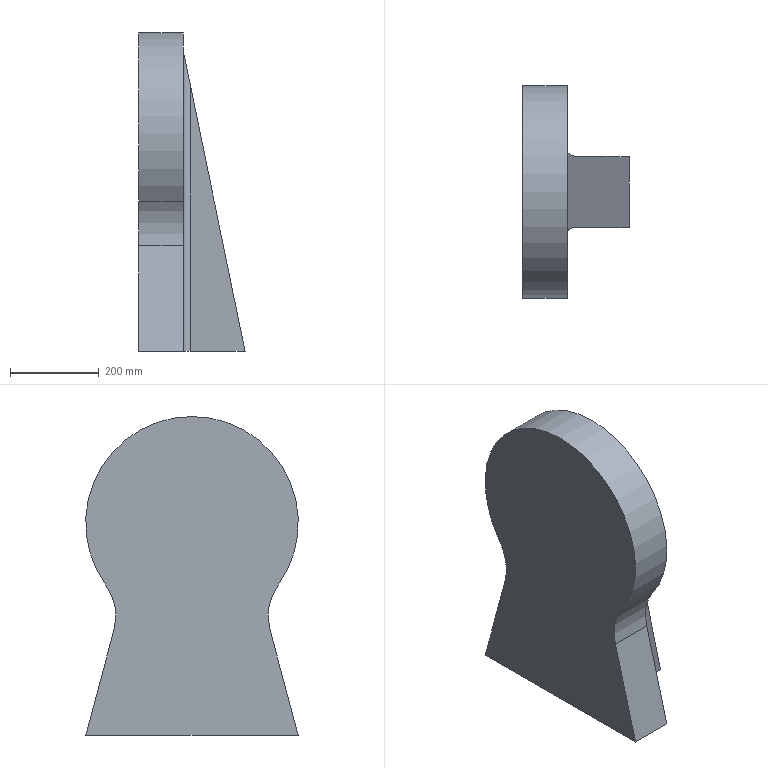Part | NX | features DATUM_CSYS 3, BLEND 2, EXTRUDE 2, SKETCH 2, CYLINDER 1 | 1 solid | 14 faces | box 240 x 480 x 720 mm | volume 36580765 mm3 | plane 8 | cylinder 6 | commonest cylinder face diameters 32 x3 240 x2 480 x1
STEP:
#1=CARTESIAN_POINT('',(100.,-96.,681.63));
#2=VERTEX_POINT('',#1);
#3=CARTESIAN_POINT('',(100.,96.,681.63));
#4=VERTEX_POINT('',#3);
#5=CARTESIAN_POINT('',(100.,0.,681.63));
#6=DIRECTION('',(0.,1.,0.));
#7=VECTOR('',#6,1000.);
#8=LINE('',#5,#7);
#9=EDGE_CURVE('',#2,#4,#8,.T.);
#10=ORIENTED_EDGE('',*,*,#9,.T.);
#11=CARTESIAN_POINT('',(100.,96.,0.));
#12=VERTEX_POINT('',#11);
#13=CARTESIAN_POINT('',(100.,96.,0.));
#14=DIRECTION('',(0.,0.,-1.));
#15=VECTOR('',#14,1000.);
#16=LINE('',#13,#15);
#17=EDGE_CURVE('',#4,#12,#16,.T.);
#18=ORIENTED_EDGE('',*,*,#17,.T.);
#19=CARTESIAN_POINT('',(100.,240.,0.));
#20=VERTEX_POINT('',#19);
#21=CARTESIAN_POINT('',(100.,-240.,0.));
#22=DIRECTION('',(0.,1.,0.));
#23=VECTOR('',#22,1000.);
#24=LINE('',#21,#23);
#25=EDGE_CURVE('',#12,#20,#24,.T.);
#26=ORIENTED_EDGE('',*,*,#25,.T.);
#27=CARTESIAN_POINT('',(100.,176.116,238.418));
#28=VERTEX_POINT('',#27);
#29=CARTESIAN_POINT('',(100.,240.,0.));
#30=DIRECTION('',(0.,-0.2588,0.9659));
#31=VECTOR('',#30,1000.);
#32=LINE('',#29,#31);
#33=EDGE_CURVE('',#20,#28,#32,.T.);
#34=ORIENTED_EDGE('',*,*,#33,.T.);
#35=CARTESIAN_POINT('',(100.,194.685,339.651));
#36=VERTEX_POINT('',#35);
#37=CARTESIAN_POINT('',(100.,292.027,269.476));
#38=DIRECTION('',(1.,0.,0.));
#39=DIRECTION('',(0.,0.,-1.));
#40=AXIS2_PLACEMENT_3D('',#37,#38,#39);
#41=CIRCLE('',#40,120.);
#42=EDGE_CURVE('',#28,#36,#41,.F.);
#43=ORIENTED_EDGE('',*,*,#42,.T.);
#44=CARTESIAN_POINT('',(100.,-194.685,339.651));
#45=VERTEX_POINT('',#44);
#46=CARTESIAN_POINT('',(100.,0.,480.));
#47=DIRECTION('',(-1.,0.,0.));
#48=DIRECTION('',(0.,0.,1.));
#49=AXIS2_PLACEMENT_3D('',#46,#47,#48);
#50=CIRCLE('',#49,240.);
#51=EDGE_CURVE('',#45,#36,#50,.T.);
#52=ORIENTED_EDGE('',*,*,#51,.F.);
#53=CARTESIAN_POINT('',(100.,-176.116,238.418));
#54=VERTEX_POINT('',#53);
#55=CARTESIAN_POINT('',(100.,-292.027,269.476));
#56=DIRECTION('',(1.,0.,0.));
#57=DIRECTION('',(0.,0.,-1.));
#58=AXIS2_PLACEMENT_3D('',#55,#56,#57);
#59=CIRCLE('',#58,120.);
#60=EDGE_CURVE('',#45,#54,#59,.F.);
#61=ORIENTED_EDGE('',*,*,#60,.T.);
#62=CARTESIAN_POINT('',(100.,-240.,0.));
#63=VERTEX_POINT('',#62);
#64=CARTESIAN_POINT('',(100.,-111.384,480.));
#65=DIRECTION('',(0.,-0.2588,-0.9659));
#66=VECTOR('',#65,1000.);
#67=LINE('',#64,#66);
#68=EDGE_CURVE('',#54,#63,#67,.T.);
#69=ORIENTED_EDGE('',*,*,#68,.T.);
#70=CARTESIAN_POINT('',(100.,-96.,0.));
#71=VERTEX_POINT('',#70);
#72=CARTESIAN_POINT('',(100.,-240.,0.));
#73=DIRECTION('',(0.,1.,0.));
#74=VECTOR('',#73,1000.);
#75=LINE('',#72,#74);
#76=EDGE_CURVE('',#63,#71,#75,.T.);
#77=ORIENTED_EDGE('',*,*,#76,.T.);
#78=CARTESIAN_POINT('',(100.,-96.,680.));
#79=DIRECTION('',(0.,0.,-1.));
#80=VECTOR('',#79,1000.);
#81=LINE('',#78,#80);
#82=EDGE_CURVE('',#71,#2,#81,.F.);
#83=ORIENTED_EDGE('',*,*,#82,.T.);
#84=EDGE_LOOP('',(#10,#18,#26,#34,#43,#52,#61,#69,#77,#83));
#85=FACE_BOUND('',#84,.T.);
#86=CARTESIAN_POINT('',(100.,0.,0.));
#87=DIRECTION('',(1.,0.,0.));
#88=DIRECTION('',(0.,0.,-1.));
#89=AXIS2_PLACEMENT_3D('',#86,#87,#88);
#90=PLANE('',#89);
#91=ADVANCED_FACE('',(#85),#90,.T.);
#92=ORIENTED_EDGE('',*,*,#68,.F.);
#93=CARTESIAN_POINT('',(0.,-176.116,238.418));
#94=VERTEX_POINT('',#93);
#95=CARTESIAN_POINT('',(100.,-176.116,238.418));
#96=DIRECTION('',(-1.,0.,0.));
#97=VECTOR('',#96,1000.);
#98=LINE('',#95,#97);
#99=EDGE_CURVE('',#54,#94,#98,.T.);
#100=ORIENTED_EDGE('',*,*,#99,.T.);
#101=CARTESIAN_POINT('',(0.,-240.,0.));
#102=VERTEX_POINT('',#101);
#103=CARTESIAN_POINT('',(0.,-111.384,480.));
#104=DIRECTION('',(0.,-0.2588,-0.9659));
#105=VECTOR('',#104,1000.);
#106=LINE('',#103,#105);
#107=EDGE_CURVE('',#94,#102,#106,.T.);
#108=ORIENTED_EDGE('',*,*,#107,.T.);
#109=CARTESIAN_POINT('',(100.,-240.,0.));
#110=DIRECTION('',(-1.,0.,0.));
#111=VECTOR('',#110,1000.);
#112=LINE('',#109,#111);
#113=EDGE_CURVE('',#63,#102,#112,.T.);
#114=ORIENTED_EDGE('',*,*,#113,.F.);
#115=EDGE_LOOP('',(#92,#100,#108,#114));
#116=FACE_BOUND('',#115,.T.);
#117=CARTESIAN_POINT('',(100.,-111.384,480.));
#118=DIRECTION('',(0.,0.9659,-0.2588));
#119=DIRECTION('',(0.,0.2588,0.9659));
#120=AXIS2_PLACEMENT_3D('',#117,#118,#119);
#121=PLANE('',#120);
#122=ADVANCED_FACE('',(#116),#121,.F.);
#123=CARTESIAN_POINT('',(0.,240.,0.));
#124=VERTEX_POINT('',#123);
#125=CARTESIAN_POINT('',(0.,-240.,0.));
#126=DIRECTION('',(0.,1.,0.));
#127=VECTOR('',#126,1000.);
#128=LINE('',#125,#127);
#129=EDGE_CURVE('',#102,#124,#128,.T.);
#130=ORIENTED_EDGE('',*,*,#129,.T.);
#131=CARTESIAN_POINT('',(100.,240.,0.));
#132=DIRECTION('',(-1.,0.,0.));
#133=VECTOR('',#132,1000.);
#134=LINE('',#131,#133);
#135=EDGE_CURVE('',#20,#124,#134,.T.);
#136=ORIENTED_EDGE('',*,*,#135,.F.);
#137=ORIENTED_EDGE('',*,*,#25,.F.);
#138=CARTESIAN_POINT('',(116.,80.,0.));
#139=VERTEX_POINT('',#138);
#140=CARTESIAN_POINT('',(116.,96.,0.));
#141=DIRECTION('',(0.,0.,1.));
#142=DIRECTION('',(1.,0.,0.));
#143=AXIS2_PLACEMENT_3D('',#140,#141,#142);
#144=CIRCLE('',#143,16.);
#145=EDGE_CURVE('',#12,#139,#144,.T.);
#146=ORIENTED_EDGE('',*,*,#145,.T.);
#147=CARTESIAN_POINT('',(240.,80.,0.));
#148=VERTEX_POINT('',#147);
#149=CARTESIAN_POINT('',(100.,80.,0.));
#150=DIRECTION('',(1.,0.,0.));
#151=VECTOR('',#150,1000.);
#152=LINE('',#149,#151);
#153=EDGE_CURVE('',#139,#148,#152,.T.);
#154=ORIENTED_EDGE('',*,*,#153,.T.);
#155=CARTESIAN_POINT('',(240.,-80.,0.));
#156=VERTEX_POINT('',#155);
#157=CARTESIAN_POINT('',(240.,-80.,0.));
#158=DIRECTION('',(0.,1.,0.));
#159=VECTOR('',#158,1000.);
#160=LINE('',#157,#159);
#161=EDGE_CURVE('',#156,#148,#160,.T.);
#162=ORIENTED_EDGE('',*,*,#161,.F.);
#163=CARTESIAN_POINT('',(116.,-80.,0.));
#164=VERTEX_POINT('',#163);
#165=CARTESIAN_POINT('',(100.,-80.,0.));
#166=DIRECTION('',(1.,0.,0.));
#167=VECTOR('',#166,1000.);
#168=LINE('',#165,#167);
#169=EDGE_CURVE('',#164,#156,#168,.T.);
#170=ORIENTED_EDGE('',*,*,#169,.F.);
#171=CARTESIAN_POINT('',(116.,-96.,0.));
#172=DIRECTION('',(0.,0.,1.));
#173=DIRECTION('',(1.,0.,0.));
#174=AXIS2_PLACEMENT_3D('',#171,#172,#173);
#175=CIRCLE('',#174,16.);
#176=EDGE_CURVE('',#164,#71,#175,.T.);
#177=ORIENTED_EDGE('',*,*,#176,.T.);
#178=ORIENTED_EDGE('',*,*,#76,.F.);
#179=ORIENTED_EDGE('',*,*,#113,.T.);
#180=EDGE_LOOP('',(#130,#136,#137,#146,#154,#162,#170,#177,#178,#179));
#181=FACE_BOUND('',#180,.T.);
#182=CARTESIAN_POINT('',(100.,-240.,0.));
#183=DIRECTION('',(0.,0.,1.));
#184=DIRECTION('',(1.,0.,0.));
#185=AXIS2_PLACEMENT_3D('',#182,#183,#184);
#186=PLANE('',#185);
#187=ADVANCED_FACE('',(#181),#186,.F.);
#188=CARTESIAN_POINT('',(0.,176.116,238.418));
#189=VERTEX_POINT('',#188);
#190=CARTESIAN_POINT('',(0.,240.,0.));
#191=DIRECTION('',(0.,-0.2588,0.9659));
#192=VECTOR('',#191,1000.);
#193=LINE('',#190,#192);
#194=EDGE_CURVE('',#124,#189,#193,.T.);
#195=ORIENTED_EDGE('',*,*,#194,.T.);
#196=CARTESIAN_POINT('',(100.,176.116,238.418));
#197=DIRECTION('',(-1.,0.,0.));
#198=VECTOR('',#197,1000.);
#199=LINE('',#196,#198);
#200=EDGE_CURVE('',#189,#28,#199,.F.);
#201=ORIENTED_EDGE('',*,*,#200,.T.);
#202=ORIENTED_EDGE('',*,*,#33,.F.);
#203=ORIENTED_EDGE('',*,*,#135,.T.);
#204=EDGE_LOOP('',(#195,#201,#202,#203));
#205=FACE_BOUND('',#204,.T.);
#206=CARTESIAN_POINT('',(100.,240.,0.));
#207=DIRECTION('',(0.,-0.9659,-0.2588));
#208=DIRECTION('',(0.,0.2588,-0.9659));
#209=AXIS2_PLACEMENT_3D('',#206,#207,#208);
#210=PLANE('',#209);
#211=ADVANCED_FACE('',(#205),#210,.F.);
#212=ORIENTED_EDGE('',*,*,#107,.F.);
#213=CARTESIAN_POINT('',(0.,-194.685,339.651));
#214=VERTEX_POINT('',#213);
#215=CARTESIAN_POINT('',(0.,-292.027,269.476));
#216=DIRECTION('',(1.,0.,0.));
#217=DIRECTION('',(0.,0.,-1.));
#218=AXIS2_PLACEMENT_3D('',#215,#216,#217);
#219=CIRCLE('',#218,120.);
#220=EDGE_CURVE('',#94,#214,#219,.T.);
#221=ORIENTED_EDGE('',*,*,#220,.T.);
#222=CARTESIAN_POINT('',(0.,194.685,339.651));
#223=VERTEX_POINT('',#222);
#224=CARTESIAN_POINT('',(0.,0.,480.));
#225=DIRECTION('',(1.,0.,0.));
#226=DIRECTION('',(0.,0.,1.));
#227=AXIS2_PLACEMENT_3D('',#224,#225,#226);
#228=CIRCLE('',#227,240.);
#229=EDGE_CURVE('',#223,#214,#228,.T.);
#230=ORIENTED_EDGE('',*,*,#229,.F.);
#231=CARTESIAN_POINT('',(0.,292.027,269.476));
#232=DIRECTION('',(1.,0.,0.));
#233=DIRECTION('',(0.,0.,-1.));
#234=AXIS2_PLACEMENT_3D('',#231,#232,#233);
#235=CIRCLE('',#234,120.);
#236=EDGE_CURVE('',#223,#189,#235,.T.);
#237=ORIENTED_EDGE('',*,*,#236,.T.);
#238=ORIENTED_EDGE('',*,*,#194,.F.);
#239=ORIENTED_EDGE('',*,*,#129,.F.);
#240=EDGE_LOOP('',(#212,#221,#230,#237,#238,#239));
#241=FACE_BOUND('',#240,.T.);
#242=CARTESIAN_POINT('',(0.,0.,0.));
#243=DIRECTION('',(1.,0.,0.));
#244=DIRECTION('',(0.,0.,-1.));
#245=AXIS2_PLACEMENT_3D('',#242,#243,#244);
#246=PLANE('',#245);
#247=ADVANCED_FACE('',(#241),#246,.F.);
#248=ORIENTED_EDGE('',*,*,#51,.T.);
#249=CARTESIAN_POINT('',(100.,194.685,339.651));
#250=DIRECTION('',(-1.,0.,0.));
#251=VECTOR('',#250,1000.);
#252=LINE('',#249,#251);
#253=EDGE_CURVE('',#36,#223,#252,.T.);
#254=ORIENTED_EDGE('',*,*,#253,.T.);
#255=ORIENTED_EDGE('',*,*,#229,.T.);
#256=CARTESIAN_POINT('',(100.,-194.685,339.651));
#257=DIRECTION('',(-1.,0.,0.));
#258=VECTOR('',#257,1000.);
#259=LINE('',#256,#258);
#260=EDGE_CURVE('',#214,#45,#259,.F.);
#261=ORIENTED_EDGE('',*,*,#260,.T.);
#262=EDGE_LOOP('',(#248,#254,#255,#261));
#263=FACE_BOUND('',#262,.T.);
#264=CARTESIAN_POINT('',(100.,0.,480.));
#265=DIRECTION('',(-1.,0.,0.));
#266=DIRECTION('',(0.,0.,1.));
#267=AXIS2_PLACEMENT_3D('',#264,#265,#266);
#268=CYLINDRICAL_SURFACE('',#267,240.);
#269=ADVANCED_FACE('',(#263),#268,.T.);
#270=CARTESIAN_POINT('',(116.,80.,602.286));
#271=VERTEX_POINT('',#270);
#272=CARTESIAN_POINT('',(240.,80.,0.));
#273=DIRECTION('',(-0.2017,0.,0.9795));
#274=VECTOR('',#273,1000.);
#275=LINE('',#272,#274);
#276=EDGE_CURVE('',#148,#271,#275,.T.);
#277=ORIENTED_EDGE('',*,*,#276,.T.);
#278=CARTESIAN_POINT('',(100.329,92.774,678.404));
#279=VERTEX_POINT('',#278);
#280=CARTESIAN_POINT('',(116.,96.,602.286));
#281=DIRECTION('',(-0.9795,0.,-0.2017));
#282=DIRECTION('',(0.2017,0.,-0.9795));
#283=AXIS2_PLACEMENT_3D('',#280,#281,#282);
#284=ELLIPSE('',#283,79.344,16.);
#285=EDGE_CURVE('',#271,#279,#284,.T.);
#286=ORIENTED_EDGE('',*,*,#285,.T.);
#287=CARTESIAN_POINT('',(100.329,-92.774,678.404));
#288=VERTEX_POINT('',#287);
#289=CARTESIAN_POINT('',(100.329,-80.,678.404));
#290=DIRECTION('',(0.,1.,0.));
#291=VECTOR('',#290,1000.);
#292=LINE('',#289,#291);
#293=EDGE_CURVE('',#279,#288,#292,.F.);
#294=ORIENTED_EDGE('',*,*,#293,.T.);
#295=CARTESIAN_POINT('',(116.,-80.,602.286));
#296=VERTEX_POINT('',#295);
#297=CARTESIAN_POINT('',(116.,-96.,602.286));
#298=DIRECTION('',(-0.9795,0.,-0.2017));
#299=DIRECTION('',(-0.2017,0.,0.9795));
#300=AXIS2_PLACEMENT_3D('',#297,#298,#299);
#301=ELLIPSE('',#300,79.344,16.);
#302=EDGE_CURVE('',#288,#296,#301,.T.);
#303=ORIENTED_EDGE('',*,*,#302,.T.);
#304=CARTESIAN_POINT('',(240.,-80.,0.));
#305=DIRECTION('',(-0.2017,0.,0.9795));
#306=VECTOR('',#305,1000.);
#307=LINE('',#304,#306);
#308=EDGE_CURVE('',#156,#296,#307,.T.);
#309=ORIENTED_EDGE('',*,*,#308,.F.);
#310=ORIENTED_EDGE('',*,*,#161,.T.);
#311=EDGE_LOOP('',(#277,#286,#294,#303,#309,#310));
#312=FACE_BOUND('',#311,.T.);
#313=CARTESIAN_POINT('',(240.,-80.,0.));
#314=DIRECTION('',(-0.9795,0.,-0.2017));
#315=DIRECTION('',(-0.2017,0.,0.9795));
#316=AXIS2_PLACEMENT_3D('',#313,#314,#315);
#317=PLANE('',#316);
#318=ADVANCED_FACE('',(#312),#317,.F.);
#319=ORIENTED_EDGE('',*,*,#308,.T.);
#320=CARTESIAN_POINT('',(116.,-80.,0.));
#321=DIRECTION('',(0.,0.,-1.));
#322=VECTOR('',#321,1000.);
#323=LINE('',#320,#322);
#324=EDGE_CURVE('',#296,#164,#323,.T.);
#325=ORIENTED_EDGE('',*,*,#324,.T.);
#326=ORIENTED_EDGE('',*,*,#169,.T.);
#327=EDGE_LOOP('',(#319,#325,#326));
#328=FACE_BOUND('',#327,.T.);
#329=CARTESIAN_POINT('',(0.,-80.,0.));
#330=DIRECTION('',(0.,-1.,0.));
#331=DIRECTION('',(0.,0.,-1.));
#332=AXIS2_PLACEMENT_3D('',#329,#330,#331);
#333=PLANE('',#332);
#334=ADVANCED_FACE('',(#328),#333,.T.);
#335=ORIENTED_EDGE('',*,*,#153,.F.);
#336=CARTESIAN_POINT('',(116.,80.,0.));
#337=DIRECTION('',(0.,0.,-1.));
#338=VECTOR('',#337,1000.);
#339=LINE('',#336,#338);
#340=EDGE_CURVE('',#139,#271,#339,.F.);
#341=ORIENTED_EDGE('',*,*,#340,.T.);
#342=ORIENTED_EDGE('',*,*,#276,.F.);
#343=EDGE_LOOP('',(#335,#341,#342));
#344=FACE_BOUND('',#343,.T.);
#345=CARTESIAN_POINT('',(0.,80.,0.));
#346=DIRECTION('',(0.,-1.,0.));
#347=DIRECTION('',(0.,0.,-1.));
#348=AXIS2_PLACEMENT_3D('',#345,#346,#347);
#349=PLANE('',#348);
#350=ADVANCED_FACE('',(#344),#349,.F.);
#351=ORIENTED_EDGE('',*,*,#324,.F.);
#352=ORIENTED_EDGE('',*,*,#302,.F.);
#353=CARTESIAN_POINT('',(116.,-96.,681.63));
#354=DIRECTION('',(0.,0.7071,0.7071));
#355=DIRECTION('',(0.,-0.7071,0.7071));
#356=AXIS2_PLACEMENT_3D('',#353,#354,#355);
#357=ELLIPSE('',#356,22.627,16.);
#358=EDGE_CURVE('',#2,#288,#357,.F.);
#359=ORIENTED_EDGE('',*,*,#358,.F.);
#360=ORIENTED_EDGE('',*,*,#82,.F.);
#361=ORIENTED_EDGE('',*,*,#176,.F.);
#362=EDGE_LOOP('',(#351,#352,#359,#360,#361));
#363=FACE_BOUND('',#362,.T.);
#364=CARTESIAN_POINT('',(116.,-96.,0.));
#365=DIRECTION('',(0.,0.,1.));
#366=DIRECTION('',(1.,0.,0.));
#367=AXIS2_PLACEMENT_3D('',#364,#365,#366);
#368=CYLINDRICAL_SURFACE('',#367,16.);
#369=ADVANCED_FACE('',(#363),#368,.F.);
#370=ORIENTED_EDGE('',*,*,#145,.F.);
#371=ORIENTED_EDGE('',*,*,#17,.F.);
#372=CARTESIAN_POINT('',(116.,96.,681.63));
#373=DIRECTION('',(0.,0.7071,-0.7071));
#374=DIRECTION('',(0.,-0.7071,-0.7071));
#375=AXIS2_PLACEMENT_3D('',#372,#373,#374);
#376=ELLIPSE('',#375,22.627,16.);
#377=EDGE_CURVE('',#279,#4,#376,.T.);
#378=ORIENTED_EDGE('',*,*,#377,.F.);
#379=ORIENTED_EDGE('',*,*,#285,.F.);
#380=ORIENTED_EDGE('',*,*,#340,.F.);
#381=EDGE_LOOP('',(#370,#371,#378,#379,#380));
#382=FACE_BOUND('',#381,.T.);
#383=CARTESIAN_POINT('',(116.,96.,0.));
#384=DIRECTION('',(0.,0.,-1.));
#385=DIRECTION('',(-1.,0.,0.));
#386=AXIS2_PLACEMENT_3D('',#383,#384,#385);
#387=CYLINDRICAL_SURFACE('',#386,16.);
#388=ADVANCED_FACE('',(#382),#387,.F.);
#389=ORIENTED_EDGE('',*,*,#358,.T.);
#390=ORIENTED_EDGE('',*,*,#293,.F.);
#391=ORIENTED_EDGE('',*,*,#377,.T.);
#392=ORIENTED_EDGE('',*,*,#9,.F.);
#393=EDGE_LOOP('',(#389,#390,#391,#392));
#394=FACE_BOUND('',#393,.T.);
#395=CARTESIAN_POINT('',(116.,0.,681.63));
#396=DIRECTION('',(0.,1.,0.));
#397=DIRECTION('',(0.,0.,1.));
#398=AXIS2_PLACEMENT_3D('',#395,#396,#397);
#399=CYLINDRICAL_SURFACE('',#398,16.);
#400=ADVANCED_FACE('',(#394),#399,.F.);
#401=ORIENTED_EDGE('',*,*,#236,.F.);
#402=ORIENTED_EDGE('',*,*,#253,.F.);
#403=ORIENTED_EDGE('',*,*,#42,.F.);
#404=ORIENTED_EDGE('',*,*,#200,.F.);
#405=EDGE_LOOP('',(#401,#402,#403,#404));
#406=FACE_BOUND('',#405,.T.);
#407=CARTESIAN_POINT('',(100.,292.027,269.476));
#408=DIRECTION('',(-1.,0.,0.));
#409=DIRECTION('',(0.,0.,1.));
#410=AXIS2_PLACEMENT_3D('',#407,#408,#409);
#411=CYLINDRICAL_SURFACE('',#410,120.);
#412=ADVANCED_FACE('',(#406),#411,.F.);
#413=ORIENTED_EDGE('',*,*,#60,.F.);
#414=ORIENTED_EDGE('',*,*,#260,.F.);
#415=ORIENTED_EDGE('',*,*,#220,.F.);
#416=ORIENTED_EDGE('',*,*,#99,.F.);
#417=EDGE_LOOP('',(#413,#414,#415,#416));
#418=FACE_BOUND('',#417,.T.);
#419=CARTESIAN_POINT('',(100.,-292.027,269.476));
#420=DIRECTION('',(-1.,0.,0.));
#421=DIRECTION('',(0.,0.,1.));
#422=AXIS2_PLACEMENT_3D('',#419,#420,#421);
#423=CYLINDRICAL_SURFACE('',#422,120.);
#424=ADVANCED_FACE('',(#418),#423,.F.);
#425=CLOSED_SHELL('',(#91,#122,#187,#211,#247,#269,#318,#334,#350,#369,#388,#400,#412,#424));
#426=MANIFOLD_SOLID_BREP('',#425);
#427=(LENGTH_UNIT()NAMED_UNIT(*)SI_UNIT(.MILLI.,.METRE.));
#428=UNCERTAINTY_MEASURE_WITH_UNIT(LENGTH_MEASURE(0.00001),#427,'','');
#429=(NAMED_UNIT(*)PLANE_ANGLE_UNIT()SI_UNIT($,.RADIAN.));
#430=(NAMED_UNIT(*)SI_UNIT($,.STERADIAN.)SOLID_ANGLE_UNIT());
#431=(GEOMETRIC_REPRESENTATION_CONTEXT(3)GLOBAL_UNCERTAINTY_ASSIGNED_CONTEXT((#428))GLOBAL_UNIT_ASSIGNED_CONTEXT((#427,#429,#430))REPRESENTATION_CONTEXT('',''));
#432=ADVANCED_BREP_SHAPE_REPRESENTATION('',(#426),#431);